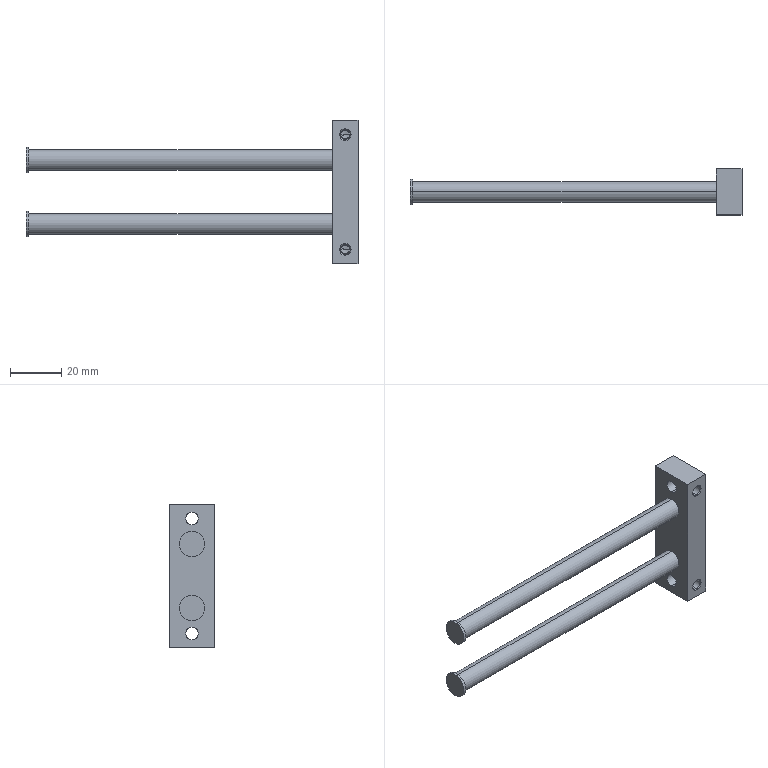Part | NX | 1 solid | 87 faces | box 130 x 18 x 56 mm | volume 21300 mm3 | cylinder 34 | plane 31 | cone 22 | commonest cylinder face diameters 3.4 x8 4 x8 5 x6 8 x4 10 x4 8.5 x2